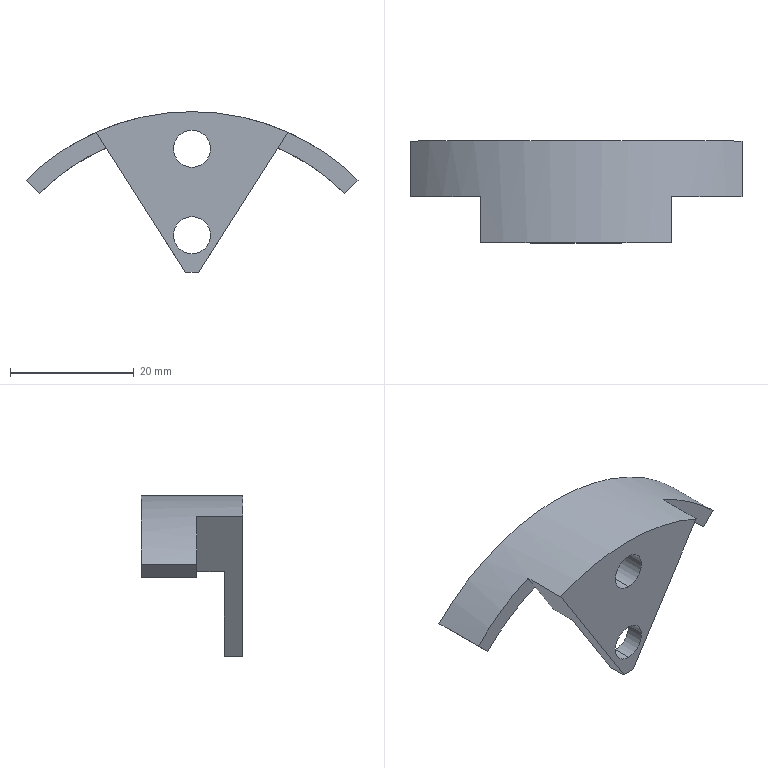Part | STEP file | Guide wheel mechanism revised.sldasm-Part-479 | 1 solid | 18 faces | box 53.74 x 16.5 x 26 mm | volume 3811 mm3 | plane 11 | cylinder 7 | commonest cylinder face diameters 6 x4 55 x1 70 x1 76 x1
STEP:
#1=CARTESIAN_POINT('',(0.,7.5,29.));
#2=VERTEX_POINT('',#1);
#3=CARTESIAN_POINT('',(0.,7.5,35.));
#4=VERTEX_POINT('',#3);
#5=CARTESIAN_POINT('',(0.,7.5,32.));
#6=DIRECTION('',(0.,1.,0.));
#7=DIRECTION('',(0.,0.,1.));
#8=AXIS2_PLACEMENT_3D('',#5,#6,#7);
#9=CIRCLE('',#8,3.);
#10=EDGE_CURVE('',#2,#4,#9,.T.);
#11=ORIENTED_EDGE('',*,*,#10,.T.);
#12=CARTESIAN_POINT('',(0.,0.,35.));
#13=VERTEX_POINT('',#12);
#14=CARTESIAN_POINT('',(0.,3.,35.));
#15=DIRECTION('',(0.,-1.,0.));
#16=VECTOR('',#15,1000.);
#17=LINE('',#14,#16);
#18=EDGE_CURVE('',#4,#13,#17,.T.);
#19=ORIENTED_EDGE('',*,*,#18,.T.);
#20=CARTESIAN_POINT('',(0.,0.,29.));
#21=VERTEX_POINT('',#20);
#22=CARTESIAN_POINT('',(0.,0.,32.));
#23=DIRECTION('',(0.,1.,0.));
#24=DIRECTION('',(0.,0.,1.));
#25=AXIS2_PLACEMENT_3D('',#22,#23,#24);
#26=CIRCLE('',#25,3.);
#27=EDGE_CURVE('',#21,#13,#26,.T.);
#28=ORIENTED_EDGE('',*,*,#27,.F.);
#29=CARTESIAN_POINT('',(0.,3.,29.));
#30=DIRECTION('',(0.,-1.,0.));
#31=VECTOR('',#30,1000.);
#32=LINE('',#29,#31);
#33=EDGE_CURVE('',#2,#21,#32,.T.);
#34=ORIENTED_EDGE('',*,*,#33,.F.);
#35=EDGE_LOOP('',(#11,#19,#28,#34));
#36=FACE_OUTER_BOUND('',#35,.T.);
#37=CARTESIAN_POINT('',(0.,3.,32.));
#38=DIRECTION('',(0.,-1.,0.));
#39=DIRECTION('',(0.,0.,-1.));
#40=AXIS2_PLACEMENT_3D('',#37,#38,#39);
#41=CYLINDRICAL_SURFACE('',#40,3.);
#42=ADVANCED_FACE('',(#36),#41,.F.);
#43=CARTESIAN_POINT('',(0.,3.,15.));
#44=VERTEX_POINT('',#43);
#45=CARTESIAN_POINT('',(0.,3.,21.));
#46=VERTEX_POINT('',#45);
#47=CARTESIAN_POINT('',(0.,3.,18.));
#48=DIRECTION('',(0.,1.,0.));
#49=DIRECTION('',(0.,0.,1.));
#50=AXIS2_PLACEMENT_3D('',#47,#48,#49);
#51=CIRCLE('',#50,3.);
#52=EDGE_CURVE('',#44,#46,#51,.T.);
#53=ORIENTED_EDGE('',*,*,#52,.T.);
#54=CARTESIAN_POINT('',(0.,0.,21.));
#55=VERTEX_POINT('',#54);
#56=CARTESIAN_POINT('',(0.,3.,21.));
#57=DIRECTION('',(0.,-1.,0.));
#58=VECTOR('',#57,1000.);
#59=LINE('',#56,#58);
#60=EDGE_CURVE('',#46,#55,#59,.T.);
#61=ORIENTED_EDGE('',*,*,#60,.T.);
#62=CARTESIAN_POINT('',(0.,0.,15.));
#63=VERTEX_POINT('',#62);
#64=CARTESIAN_POINT('',(0.,0.,18.));
#65=DIRECTION('',(0.,1.,0.));
#66=DIRECTION('',(0.,0.,1.));
#67=AXIS2_PLACEMENT_3D('',#64,#65,#66);
#68=CIRCLE('',#67,3.);
#69=EDGE_CURVE('',#63,#55,#68,.T.);
#70=ORIENTED_EDGE('',*,*,#69,.F.);
#71=CARTESIAN_POINT('',(0.,3.,15.));
#72=DIRECTION('',(0.,-1.,0.));
#73=VECTOR('',#72,1000.);
#74=LINE('',#71,#73);
#75=EDGE_CURVE('',#44,#63,#74,.T.);
#76=ORIENTED_EDGE('',*,*,#75,.F.);
#77=EDGE_LOOP('',(#53,#61,#70,#76));
#78=FACE_OUTER_BOUND('',#77,.T.);
#79=CARTESIAN_POINT('',(0.,3.,18.));
#80=DIRECTION('',(0.,-1.,0.));
#81=DIRECTION('',(0.,0.,-1.));
#82=AXIS2_PLACEMENT_3D('',#79,#80,#81);
#83=CYLINDRICAL_SURFACE('',#82,3.);
#84=ADVANCED_FACE('',(#78),#83,.F.);
#85=CARTESIAN_POINT('',(9.775,3.,25.704));
#86=VERTEX_POINT('',#85);
#87=CARTESIAN_POINT('',(-9.775,3.,25.704));
#88=VERTEX_POINT('',#87);
#89=CARTESIAN_POINT('',(0.,3.,0.));
#90=DIRECTION('',(0.,-1.,0.));
#91=DIRECTION('',(0.,0.,1.));
#92=AXIS2_PLACEMENT_3D('',#89,#90,#91);
#93=CIRCLE('',#92,27.5);
#94=EDGE_CURVE('',#86,#88,#93,.T.);
#95=ORIENTED_EDGE('',*,*,#94,.F.);
#96=CARTESIAN_POINT('',(1.044,3.,12.));
#97=VERTEX_POINT('',#96);
#98=CARTESIAN_POINT('',(1.044,3.,12.));
#99=DIRECTION('',(-0.5373,0.,-0.8434));
#100=VECTOR('',#99,1000.);
#101=LINE('',#98,#100);
#102=EDGE_CURVE('',#86,#97,#101,.T.);
#103=ORIENTED_EDGE('',*,*,#102,.T.);
#104=CARTESIAN_POINT('',(-1.044,3.,12.));
#105=VERTEX_POINT('',#104);
#106=CARTESIAN_POINT('',(1.044,3.,12.));
#107=DIRECTION('',(-1.,0.,0.));
#108=VECTOR('',#107,1000.);
#109=LINE('',#106,#108);
#110=EDGE_CURVE('',#97,#105,#109,.T.);
#111=ORIENTED_EDGE('',*,*,#110,.T.);
#112=CARTESIAN_POINT('',(-1.044,3.,12.));
#113=DIRECTION('',(-0.5373,0.,0.8434));
#114=VECTOR('',#113,1000.);
#115=LINE('',#112,#114);
#116=EDGE_CURVE('',#105,#88,#115,.T.);
#117=ORIENTED_EDGE('',*,*,#116,.T.);
#118=EDGE_LOOP('',(#95,#103,#111,#117));
#119=FACE_OUTER_BOUND('',#118,.T.);
#120=ORIENTED_EDGE('',*,*,#52,.F.);
#121=CARTESIAN_POINT('',(0.,3.,18.));
#122=DIRECTION('',(0.,1.,0.));
#123=DIRECTION('',(0.,0.,1.));
#124=AXIS2_PLACEMENT_3D('',#121,#122,#123);
#125=CIRCLE('',#124,3.);
#126=EDGE_CURVE('',#46,#44,#125,.T.);
#127=ORIENTED_EDGE('',*,*,#126,.F.);
#128=EDGE_LOOP('',(#120,#127));
#129=FACE_BOUND('',#128,.T.);
#130=CARTESIAN_POINT('',(0.,3.,0.));
#131=DIRECTION('',(0.,1.,0.));
#132=DIRECTION('',(0.,0.,1.));
#133=AXIS2_PLACEMENT_3D('',#130,#131,#132);
#134=PLANE('',#133);
#135=ADVANCED_FACE('',(#119,#129),#134,.T.);
#136=ORIENTED_EDGE('',*,*,#69,.T.);
#137=CARTESIAN_POINT('',(0.,0.,18.));
#138=DIRECTION('',(0.,1.,0.));
#139=DIRECTION('',(0.,0.,1.));
#140=AXIS2_PLACEMENT_3D('',#137,#138,#139);
#141=CIRCLE('',#140,3.);
#142=EDGE_CURVE('',#55,#63,#141,.T.);
#143=ORIENTED_EDGE('',*,*,#142,.T.);
#144=EDGE_LOOP('',(#136,#143));
#145=FACE_BOUND('',#144,.T.);
#146=CARTESIAN_POINT('',(1.044,0.,12.));
#147=VERTEX_POINT('',#146);
#148=CARTESIAN_POINT('',(-1.044,0.,12.));
#149=VERTEX_POINT('',#148);
#150=CARTESIAN_POINT('',(1.044,0.,12.));
#151=DIRECTION('',(-1.,0.,0.));
#152=VECTOR('',#151,1000.);
#153=LINE('',#150,#152);
#154=EDGE_CURVE('',#147,#149,#153,.T.);
#155=ORIENTED_EDGE('',*,*,#154,.F.);
#156=CARTESIAN_POINT('',(15.502,0.,34.694));
#157=VERTEX_POINT('',#156);
#158=CARTESIAN_POINT('',(1.044,0.,12.));
#159=DIRECTION('',(-0.5373,0.,-0.8434));
#160=VECTOR('',#159,1000.);
#161=LINE('',#158,#160);
#162=EDGE_CURVE('',#157,#147,#161,.T.);
#163=ORIENTED_EDGE('',*,*,#162,.F.);
#164=CARTESIAN_POINT('',(-15.502,0.,34.694));
#165=VERTEX_POINT('',#164);
#166=CARTESIAN_POINT('',(0.,0.,0.));
#167=DIRECTION('',(0.,1.,0.));
#168=DIRECTION('',(0.,0.,1.));
#169=AXIS2_PLACEMENT_3D('',#166,#167,#168);
#170=CIRCLE('',#169,38.);
#171=EDGE_CURVE('',#165,#157,#170,.T.);
#172=ORIENTED_EDGE('',*,*,#171,.F.);
#173=CARTESIAN_POINT('',(-1.044,0.,12.));
#174=DIRECTION('',(-0.5373,0.,0.8434));
#175=VECTOR('',#174,1000.);
#176=LINE('',#173,#175);
#177=EDGE_CURVE('',#149,#165,#176,.T.);
#178=ORIENTED_EDGE('',*,*,#177,.F.);
#179=EDGE_LOOP('',(#155,#163,#172,#178));
#180=FACE_OUTER_BOUND('',#179,.T.);
#181=ORIENTED_EDGE('',*,*,#27,.T.);
#182=CARTESIAN_POINT('',(0.,0.,32.));
#183=DIRECTION('',(0.,1.,0.));
#184=DIRECTION('',(0.,0.,1.));
#185=AXIS2_PLACEMENT_3D('',#182,#183,#184);
#186=CIRCLE('',#185,3.);
#187=EDGE_CURVE('',#13,#21,#186,.T.);
#188=ORIENTED_EDGE('',*,*,#187,.T.);
#189=EDGE_LOOP('',(#181,#188));
#190=FACE_BOUND('',#189,.T.);
#191=CARTESIAN_POINT('',(0.,0.,0.));
#192=DIRECTION('',(0.,1.,0.));
#193=DIRECTION('',(0.,0.,1.));
#194=AXIS2_PLACEMENT_3D('',#191,#192,#193);
#195=PLANE('',#194);
#196=ADVANCED_FACE('',(#145,#180,#190),#195,.F.);
#197=ORIENTED_EDGE('',*,*,#154,.T.);
#198=CARTESIAN_POINT('',(-1.044,3.,12.));
#199=DIRECTION('',(0.,-1.,0.));
#200=VECTOR('',#199,1000.);
#201=LINE('',#198,#200);
#202=EDGE_CURVE('',#105,#149,#201,.T.);
#203=ORIENTED_EDGE('',*,*,#202,.F.);
#204=ORIENTED_EDGE('',*,*,#110,.F.);
#205=CARTESIAN_POINT('',(1.044,3.,12.));
#206=DIRECTION('',(0.,-1.,0.));
#207=VECTOR('',#206,1000.);
#208=LINE('',#205,#207);
#209=EDGE_CURVE('',#97,#147,#208,.T.);
#210=ORIENTED_EDGE('',*,*,#209,.T.);
#211=EDGE_LOOP('',(#197,#203,#204,#210));
#212=FACE_OUTER_BOUND('',#211,.T.);
#213=CARTESIAN_POINT('',(1.044,3.,12.));
#214=DIRECTION('',(0.,0.,1.));
#215=DIRECTION('',(1.,0.,0.));
#216=AXIS2_PLACEMENT_3D('',#213,#214,#215);
#217=PLANE('',#216);
#218=ADVANCED_FACE('',(#212),#217,.F.);
#219=ORIENTED_EDGE('',*,*,#177,.T.);
#220=CARTESIAN_POINT('',(-15.502,7.5,34.694));
#221=VERTEX_POINT('',#220);
#222=CARTESIAN_POINT('',(-15.502,3.,34.694));
#223=DIRECTION('',(0.,-1.,0.));
#224=VECTOR('',#223,1000.);
#225=LINE('',#222,#224);
#226=EDGE_CURVE('',#221,#165,#225,.T.);
#227=ORIENTED_EDGE('',*,*,#226,.F.);
#228=CARTESIAN_POINT('',(-13.871,7.5,32.134));
#229=VERTEX_POINT('',#228);
#230=CARTESIAN_POINT('',(-9.775,7.5,25.704));
#231=DIRECTION('',(-0.5373,0.,0.8434));
#232=VECTOR('',#231,1000.);
#233=LINE('',#230,#232);
#234=EDGE_CURVE('',#229,#221,#233,.T.);
#235=ORIENTED_EDGE('',*,*,#234,.F.);
#236=CARTESIAN_POINT('',(-9.775,7.5,25.704));
#237=VERTEX_POINT('',#236);
#238=CARTESIAN_POINT('',(-9.775,7.5,25.704));
#239=DIRECTION('',(-0.5373,0.,0.8434));
#240=VECTOR('',#239,1000.);
#241=LINE('',#238,#240);
#242=EDGE_CURVE('',#237,#229,#241,.T.);
#243=ORIENTED_EDGE('',*,*,#242,.F.);
#244=CARTESIAN_POINT('',(-9.775,7.5,25.704));
#245=DIRECTION('',(0.,-1.,0.));
#246=VECTOR('',#245,1000.);
#247=LINE('',#244,#246);
#248=EDGE_CURVE('',#237,#88,#247,.T.);
#249=ORIENTED_EDGE('',*,*,#248,.T.);
#250=ORIENTED_EDGE('',*,*,#116,.F.);
#251=ORIENTED_EDGE('',*,*,#202,.T.);
#252=EDGE_LOOP('',(#219,#227,#235,#243,#249,#250,#251));
#253=FACE_OUTER_BOUND('',#252,.T.);
#254=CARTESIAN_POINT('',(-1.044,3.,12.));
#255=DIRECTION('',(0.8434,0.,0.5373));
#256=DIRECTION('',(0.5373,0.,-0.8434));
#257=AXIS2_PLACEMENT_3D('',#254,#255,#256);
#258=PLANE('',#257);
#259=ADVANCED_FACE('',(#253),#258,.F.);
#260=ORIENTED_EDGE('',*,*,#171,.T.);
#261=CARTESIAN_POINT('',(15.502,7.5,34.694));
#262=VERTEX_POINT('',#261);
#263=CARTESIAN_POINT('',(15.502,3.,34.694));
#264=DIRECTION('',(0.,-1.,0.));
#265=VECTOR('',#264,1000.);
#266=LINE('',#263,#265);
#267=EDGE_CURVE('',#262,#157,#266,.T.);
#268=ORIENTED_EDGE('',*,*,#267,.F.);
#269=CARTESIAN_POINT('',(26.87,7.5,26.87));
#270=VERTEX_POINT('',#269);
#271=CARTESIAN_POINT('',(0.,7.5,0.));
#272=DIRECTION('',(0.,1.,0.));
#273=DIRECTION('',(0.,0.,1.));
#274=AXIS2_PLACEMENT_3D('',#271,#272,#273);
#275=CIRCLE('',#274,38.);
#276=EDGE_CURVE('',#262,#270,#275,.T.);
#277=ORIENTED_EDGE('',*,*,#276,.T.);
#278=CARTESIAN_POINT('',(26.87,16.5,26.87));
#279=VERTEX_POINT('',#278);
#280=CARTESIAN_POINT('',(26.87,16.5,26.87));
#281=DIRECTION('',(0.,-1.,0.));
#282=VECTOR('',#281,1000.);
#283=LINE('',#280,#282);
#284=EDGE_CURVE('',#279,#270,#283,.T.);
#285=ORIENTED_EDGE('',*,*,#284,.F.);
#286=CARTESIAN_POINT('',(-26.87,16.5,26.87));
#287=VERTEX_POINT('',#286);
#288=CARTESIAN_POINT('',(0.,16.5,0.));
#289=DIRECTION('',(0.,1.,0.));
#290=DIRECTION('',(0.,0.,1.));
#291=AXIS2_PLACEMENT_3D('',#288,#289,#290);
#292=CIRCLE('',#291,38.);
#293=EDGE_CURVE('',#287,#279,#292,.T.);
#294=ORIENTED_EDGE('',*,*,#293,.F.);
#295=CARTESIAN_POINT('',(-26.87,7.5,26.87));
#296=VERTEX_POINT('',#295);
#297=CARTESIAN_POINT('',(-26.87,16.5,26.87));
#298=DIRECTION('',(0.,-1.,0.));
#299=VECTOR('',#298,1000.);
#300=LINE('',#297,#299);
#301=EDGE_CURVE('',#287,#296,#300,.T.);
#302=ORIENTED_EDGE('',*,*,#301,.T.);
#303=CARTESIAN_POINT('',(0.,7.5,0.));
#304=DIRECTION('',(0.,1.,0.));
#305=DIRECTION('',(0.,0.,1.));
#306=AXIS2_PLACEMENT_3D('',#303,#304,#305);
#307=CIRCLE('',#306,38.);
#308=EDGE_CURVE('',#296,#221,#307,.T.);
#309=ORIENTED_EDGE('',*,*,#308,.T.);
#310=ORIENTED_EDGE('',*,*,#226,.T.);
#311=EDGE_LOOP('',(#260,#268,#277,#285,#294,#302,#309,#310));
#312=FACE_OUTER_BOUND('',#311,.T.);
#313=CARTESIAN_POINT('',(0.,3.,0.));
#314=DIRECTION('',(0.,-1.,0.));
#315=DIRECTION('',(0.,0.,-1.));
#316=AXIS2_PLACEMENT_3D('',#313,#314,#315);
#317=CYLINDRICAL_SURFACE('',#316,38.);
#318=ADVANCED_FACE('',(#312),#317,.T.);
#319=ORIENTED_EDGE('',*,*,#162,.T.);
#320=ORIENTED_EDGE('',*,*,#209,.F.);
#321=ORIENTED_EDGE('',*,*,#102,.F.);
#322=CARTESIAN_POINT('',(9.775,7.5,25.704));
#323=VERTEX_POINT('',#322);
#324=CARTESIAN_POINT('',(9.775,7.5,25.704));
#325=DIRECTION('',(0.,-1.,0.));
#326=VECTOR('',#325,1000.);
#327=LINE('',#324,#326);
#328=EDGE_CURVE('',#323,#86,#327,.T.);
#329=ORIENTED_EDGE('',*,*,#328,.F.);
#330=CARTESIAN_POINT('',(13.871,7.5,32.134));
#331=VERTEX_POINT('',#330);
#332=CARTESIAN_POINT('',(9.775,7.5,25.704));
#333=DIRECTION('',(-0.5373,0.,-0.8434));
#334=VECTOR('',#333,1000.);
#335=LINE('',#332,#334);
#336=EDGE_CURVE('',#331,#323,#335,.T.);
#337=ORIENTED_EDGE('',*,*,#336,.F.);
#338=CARTESIAN_POINT('',(9.775,7.5,25.704));
#339=DIRECTION('',(-0.5373,0.,-0.8434));
#340=VECTOR('',#339,1000.);
#341=LINE('',#338,#340);
#342=EDGE_CURVE('',#262,#331,#341,.T.);
#343=ORIENTED_EDGE('',*,*,#342,.F.);
#344=ORIENTED_EDGE('',*,*,#267,.T.);
#345=EDGE_LOOP('',(#319,#320,#321,#329,#337,#343,#344));
#346=FACE_OUTER_BOUND('',#345,.T.);
#347=CARTESIAN_POINT('',(1.044,3.,12.));
#348=DIRECTION('',(-0.8434,0.,0.5373));
#349=DIRECTION('',(0.5373,0.,0.8434));
#350=AXIS2_PLACEMENT_3D('',#347,#348,#349);
#351=PLANE('',#350);
#352=ADVANCED_FACE('',(#346),#351,.F.);
#353=ORIENTED_EDGE('',*,*,#60,.F.);
#354=ORIENTED_EDGE('',*,*,#126,.T.);
#355=ORIENTED_EDGE('',*,*,#75,.T.);
#356=ORIENTED_EDGE('',*,*,#142,.F.);
#357=EDGE_LOOP('',(#353,#354,#355,#356));
#358=FACE_OUTER_BOUND('',#357,.T.);
#359=CARTESIAN_POINT('',(0.,3.,18.));
#360=DIRECTION('',(0.,-1.,0.));
#361=DIRECTION('',(0.,0.,-1.));
#362=AXIS2_PLACEMENT_3D('',#359,#360,#361);
#363=CYLINDRICAL_SURFACE('',#362,3.);
#364=ADVANCED_FACE('',(#358),#363,.F.);
#365=ORIENTED_EDGE('',*,*,#18,.F.);
#366=CARTESIAN_POINT('',(0.,7.5,32.));
#367=DIRECTION('',(0.,1.,0.));
#368=DIRECTION('',(0.,0.,1.));
#369=AXIS2_PLACEMENT_3D('',#366,#367,#368);
#370=CIRCLE('',#369,3.);
#371=EDGE_CURVE('',#4,#2,#370,.T.);
#372=ORIENTED_EDGE('',*,*,#371,.T.);
#373=ORIENTED_EDGE('',*,*,#33,.T.);
#374=ORIENTED_EDGE('',*,*,#187,.F.);
#375=EDGE_LOOP('',(#365,#372,#373,#374));
#376=FACE_OUTER_BOUND('',#375,.T.);
#377=CARTESIAN_POINT('',(0.,3.,32.));
#378=DIRECTION('',(0.,-1.,0.));
#379=DIRECTION('',(0.,0.,-1.));
#380=AXIS2_PLACEMENT_3D('',#377,#378,#379);
#381=CYLINDRICAL_SURFACE('',#380,3.);
#382=ADVANCED_FACE('',(#376),#381,.F.);
#383=CARTESIAN_POINT('',(0.,7.5,0.));
#384=DIRECTION('',(0.,-1.,0.));
#385=DIRECTION('',(0.,0.,1.));
#386=AXIS2_PLACEMENT_3D('',#383,#384,#385);
#387=CIRCLE('',#386,35.);
#388=EDGE_CURVE('',#331,#4,#387,.T.);
#389=ORIENTED_EDGE('',*,*,#388,.F.);
#390=ORIENTED_EDGE('',*,*,#336,.T.);
#391=CARTESIAN_POINT('',(0.,7.5,0.));
#392=DIRECTION('',(0.,-1.,0.));
#393=DIRECTION('',(0.,0.,1.));
#394=AXIS2_PLACEMENT_3D('',#391,#392,#393);
#395=CIRCLE('',#394,27.5);
#396=EDGE_CURVE('',#323,#237,#395,.T.);
#397=ORIENTED_EDGE('',*,*,#396,.T.);
#398=ORIENTED_EDGE('',*,*,#242,.T.);
#399=CARTESIAN_POINT('',(0.,7.5,0.));
#400=DIRECTION('',(0.,-1.,0.));
#401=DIRECTION('',(0.,0.,1.));
#402=AXIS2_PLACEMENT_3D('',#399,#400,#401);
#403=CIRCLE('',#402,35.);
#404=EDGE_CURVE('',#4,#229,#403,.T.);
#405=ORIENTED_EDGE('',*,*,#404,.F.);
#406=ORIENTED_EDGE('',*,*,#10,.F.);
#407=ORIENTED_EDGE('',*,*,#371,.F.);
#408=EDGE_LOOP('',(#389,#390,#397,#398,#405,#406,#407));
#409=FACE_OUTER_BOUND('',#408,.T.);
#410=CARTESIAN_POINT('',(0.,7.5,0.));
#411=DIRECTION('',(0.,1.,0.));
#412=DIRECTION('',(0.,0.,1.));
#413=AXIS2_PLACEMENT_3D('',#410,#411,#412);
#414=PLANE('',#413);
#415=ADVANCED_FACE('',(#409),#414,.T.);
#416=ORIENTED_EDGE('',*,*,#94,.T.);
#417=ORIENTED_EDGE('',*,*,#248,.F.);
#418=ORIENTED_EDGE('',*,*,#396,.F.);
#419=ORIENTED_EDGE('',*,*,#328,.T.);
#420=EDGE_LOOP('',(#416,#417,#418,#419));
#421=FACE_OUTER_BOUND('',#420,.T.);
#422=CARTESIAN_POINT('',(0.,7.5,0.));
#423=DIRECTION('',(0.,-1.,0.));
#424=DIRECTION('',(0.,0.,-1.));
#425=AXIS2_PLACEMENT_3D('',#422,#423,#424);
#426=CYLINDRICAL_SURFACE('',#425,27.5);
#427=ADVANCED_FACE('',(#421),#426,.F.);
#428=CARTESIAN_POINT('',(-24.749,7.5,24.749));
#429=VERTEX_POINT('',#428);
#430=CARTESIAN_POINT('',(0.,7.5,0.));
#431=DIRECTION('',(0.,-1.,0.));
#432=DIRECTION('',(0.,0.,1.));
#433=AXIS2_PLACEMENT_3D('',#430,#431,#432);
#434=CIRCLE('',#433,35.);
#435=EDGE_CURVE('',#229,#429,#434,.T.);
#436=ORIENTED_EDGE('',*,*,#435,.F.);
#437=ORIENTED_EDGE('',*,*,#234,.T.);
#438=ORIENTED_EDGE('',*,*,#308,.F.);
#439=CARTESIAN_POINT('',(-24.749,7.5,24.749));
#440=DIRECTION('',(-0.7071,0.,0.7071));
#441=VECTOR('',#440,1000.);
#442=LINE('',#439,#441);
#443=EDGE_CURVE('',#429,#296,#442,.T.);
#444=ORIENTED_EDGE('',*,*,#443,.F.);
#445=EDGE_LOOP('',(#436,#437,#438,#444));
#446=FACE_OUTER_BOUND('',#445,.T.);
#447=CARTESIAN_POINT('',(0.,7.5,0.));
#448=DIRECTION('',(0.,1.,0.));
#449=DIRECTION('',(0.,0.,1.));
#450=AXIS2_PLACEMENT_3D('',#447,#448,#449);
#451=PLANE('',#450);
#452=ADVANCED_FACE('',(#446),#451,.F.);
#453=ORIENTED_EDGE('',*,*,#276,.F.);
#454=ORIENTED_EDGE('',*,*,#342,.T.);
#455=CARTESIAN_POINT('',(24.749,7.5,24.749));
#456=VERTEX_POINT('',#455);
#457=CARTESIAN_POINT('',(0.,7.5,0.));
#458=DIRECTION('',(0.,-1.,0.));
#459=DIRECTION('',(0.,0.,1.));
#460=AXIS2_PLACEMENT_3D('',#457,#458,#459);
#461=CIRCLE('',#460,35.);
#462=EDGE_CURVE('',#456,#331,#461,.T.);
#463=ORIENTED_EDGE('',*,*,#462,.F.);
#464=CARTESIAN_POINT('',(24.749,7.5,24.749));
#465=DIRECTION('',(-0.7071,0.,-0.7071));
#466=VECTOR('',#465,1000.);
#467=LINE('',#464,#466);
#468=EDGE_CURVE('',#270,#456,#467,.T.);
#469=ORIENTED_EDGE('',*,*,#468,.F.);
#470=EDGE_LOOP('',(#453,#454,#463,#469));
#471=FACE_OUTER_BOUND('',#470,.T.);
#472=CARTESIAN_POINT('',(0.,7.5,0.));
#473=DIRECTION('',(0.,1.,0.));
#474=DIRECTION('',(0.,0.,1.));
#475=AXIS2_PLACEMENT_3D('',#472,#473,#474);
#476=PLANE('',#475);
#477=ADVANCED_FACE('',(#471),#476,.F.);
#478=ORIENTED_EDGE('',*,*,#462,.T.);
#479=ORIENTED_EDGE('',*,*,#388,.T.);
#480=ORIENTED_EDGE('',*,*,#404,.T.);
#481=ORIENTED_EDGE('',*,*,#435,.T.);
#482=CARTESIAN_POINT('',(-24.749,16.5,24.749));
#483=VERTEX_POINT('',#482);
#484=CARTESIAN_POINT('',(-24.749,16.5,24.749));
#485=DIRECTION('',(0.,-1.,0.));
#486=VECTOR('',#485,1000.);
#487=LINE('',#484,#486);
#488=EDGE_CURVE('',#483,#429,#487,.T.);
#489=ORIENTED_EDGE('',*,*,#488,.F.);
#490=CARTESIAN_POINT('',(24.749,16.5,24.749));
#491=VERTEX_POINT('',#490);
#492=CARTESIAN_POINT('',(0.,16.5,0.));
#493=DIRECTION('',(0.,-1.,0.));
#494=DIRECTION('',(0.,0.,1.));
#495=AXIS2_PLACEMENT_3D('',#492,#493,#494);
#496=CIRCLE('',#495,35.);
#497=EDGE_CURVE('',#491,#483,#496,.T.);
#498=ORIENTED_EDGE('',*,*,#497,.F.);
#499=CARTESIAN_POINT('',(24.749,16.5,24.749));
#500=DIRECTION('',(0.,-1.,0.));
#501=VECTOR('',#500,1000.);
#502=LINE('',#499,#501);
#503=EDGE_CURVE('',#491,#456,#502,.T.);
#504=ORIENTED_EDGE('',*,*,#503,.T.);
#505=EDGE_LOOP('',(#478,#479,#480,#481,#489,#498,#504));
#506=FACE_OUTER_BOUND('',#505,.T.);
#507=CARTESIAN_POINT('',(0.,16.5,0.));
#508=DIRECTION('',(0.,-1.,0.));
#509=DIRECTION('',(0.,0.,-1.));
#510=AXIS2_PLACEMENT_3D('',#507,#508,#509);
#511=CYLINDRICAL_SURFACE('',#510,35.);
#512=ADVANCED_FACE('',(#506),#511,.F.);
#513=ORIENTED_EDGE('',*,*,#443,.T.);
#514=ORIENTED_EDGE('',*,*,#301,.F.);
#515=CARTESIAN_POINT('',(-24.749,16.5,24.749));
#516=DIRECTION('',(-0.7071,0.,0.7071));
#517=VECTOR('',#516,1000.);
#518=LINE('',#515,#517);
#519=EDGE_CURVE('',#483,#287,#518,.T.);
#520=ORIENTED_EDGE('',*,*,#519,.F.);
#521=ORIENTED_EDGE('',*,*,#488,.T.);
#522=EDGE_LOOP('',(#513,#514,#520,#521));
#523=FACE_OUTER_BOUND('',#522,.T.);
#524=CARTESIAN_POINT('',(-24.749,16.5,24.749));
#525=DIRECTION('',(0.7071,0.,0.7071));
#526=DIRECTION('',(0.7071,0.,-0.7071));
#527=AXIS2_PLACEMENT_3D('',#524,#525,#526);
#528=PLANE('',#527);
#529=ADVANCED_FACE('',(#523),#528,.F.);
#530=ORIENTED_EDGE('',*,*,#468,.T.);
#531=ORIENTED_EDGE('',*,*,#503,.F.);
#532=CARTESIAN_POINT('',(24.749,16.5,24.749));
#533=DIRECTION('',(-0.7071,0.,-0.7071));
#534=VECTOR('',#533,1000.);
#535=LINE('',#532,#534);
#536=EDGE_CURVE('',#279,#491,#535,.T.);
#537=ORIENTED_EDGE('',*,*,#536,.F.);
#538=ORIENTED_EDGE('',*,*,#284,.T.);
#539=EDGE_LOOP('',(#530,#531,#537,#538));
#540=FACE_OUTER_BOUND('',#539,.T.);
#541=CARTESIAN_POINT('',(24.749,16.5,24.749));
#542=DIRECTION('',(-0.7071,0.,0.7071));
#543=DIRECTION('',(0.7071,0.,0.7071));
#544=AXIS2_PLACEMENT_3D('',#541,#542,#543);
#545=PLANE('',#544);
#546=ADVANCED_FACE('',(#540),#545,.F.);
#547=ORIENTED_EDGE('',*,*,#497,.T.);
#548=ORIENTED_EDGE('',*,*,#519,.T.);
#549=ORIENTED_EDGE('',*,*,#293,.T.);
#550=ORIENTED_EDGE('',*,*,#536,.T.);
#551=EDGE_LOOP('',(#547,#548,#549,#550));
#552=FACE_OUTER_BOUND('',#551,.T.);
#553=CARTESIAN_POINT('',(0.,16.5,0.));
#554=DIRECTION('',(0.,1.,0.));
#555=DIRECTION('',(0.,0.,1.));
#556=AXIS2_PLACEMENT_3D('',#553,#554,#555);
#557=PLANE('',#556);
#558=ADVANCED_FACE('',(#552),#557,.T.);
#559=CLOSED_SHELL('',(#42,#84,#135,#196,#218,#259,#318,#352,#364,#382,#415,#427,#452,#477,#512,#529,#546,#558));
#560=MANIFOLD_SOLID_BREP('',#559);
#561=CARTESIAN_POINT('',(0.,0.,0.));
#562=DIRECTION('',(0.,0.,1.));
#563=DIRECTION('',(1.,0.,0.));
#564=AXIS2_PLACEMENT_3D('',#561,#562,#563);
#565=(LENGTH_UNIT()NAMED_UNIT(*)SI_UNIT(.MILLI.,.METRE.));
#566=UNCERTAINTY_MEASURE_WITH_UNIT(LENGTH_MEASURE(0.00001),#565,'','');
#567=(NAMED_UNIT(*)PLANE_ANGLE_UNIT()SI_UNIT($,.RADIAN.));
#568=(NAMED_UNIT(*)SI_UNIT($,.STERADIAN.)SOLID_ANGLE_UNIT());
#569=(GEOMETRIC_REPRESENTATION_CONTEXT(3)GLOBAL_UNCERTAINTY_ASSIGNED_CONTEXT((#566))GLOBAL_UNIT_ASSIGNED_CONTEXT((#565,#567,#568))REPRESENTATION_CONTEXT('',''));
#570=ADVANCED_BREP_SHAPE_REPRESENTATION('',(#560,#564),#569);